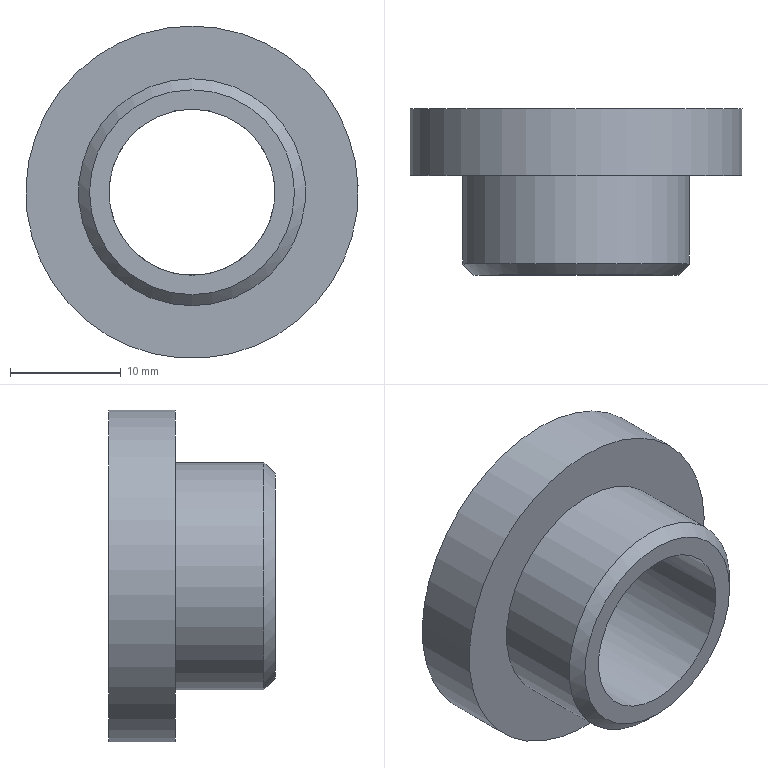Part | STEP file | HL4GZ-1.58.105 (cane-lifter cylinder pin bushing) | 1 solid | 8 faces | box 30 x 15 x 30 mm | volume 4505 mm3 | cylinder 3 | plane 3 | cone 2 | commonest cylinder face diameters 15 x1 20.5 x1 30 x1
STEP:
#1=CARTESIAN_POINT('',(0.,0.,0.));
#2=DIRECTION('',(0.,0.,1.));
#3=DIRECTION('',(1.,0.,0.));
#4=AXIS2_PLACEMENT_3D('',#1,#2,#3);
#5=CARTESIAN_POINT('',(3259.883,-564.,17.811));
#6=VERTEX_POINT('',#5);
#7=CARTESIAN_POINT('',(3259.883,-564.,10.311));
#8=DIRECTION('',(0.000001603,1.,0.000002068));
#9=DIRECTION('',(0.,-0.000002068,1.));
#10=AXIS2_PLACEMENT_3D('',#7,#8,#9);
#11=CIRCLE('',#10,7.5);
#12=CARTESIAN_POINT('',(3259.883,-564.,10.311));
#13=DIRECTION('',(0.000001603,1.,0.000002068));
#14=DIRECTION('',(0.,0.000002068,-1.));
#15=AXIS2_PLACEMENT_3D('',#12,#13,#14);
#16=CONICAL_SURFACE('',#15,7.5,0.7854);
#17=CARTESIAN_POINT('',(3.142,0.));
#18=DIRECTION('',(1.,0.));
#19=VECTOR('',#18,1.);
#20=LINE('',#17,#19);
#21=(GEOMETRIC_REPRESENTATION_CONTEXT(2)PARAMETRIC_REPRESENTATION_CONTEXT()REPRESENTATION_CONTEXT('',''));
#22=DEFINITIONAL_REPRESENTATION('',(#20),#21);
#23=PCURVE('',#16,#22);
#24=CARTESIAN_POINT('',(3259.883,-563.,10.311));
#25=DIRECTION('',(-0.000001603,-1.,-0.000002068));
#26=DIRECTION('',(0.,-0.000002068,1.));
#27=AXIS2_PLACEMENT_3D('',#24,#25,#26);
#28=CYLINDRICAL_SURFACE('',#27,7.5);
#29=CARTESIAN_POINT('',(6.283,1.));
#30=DIRECTION('',(-1.,0.));
#31=VECTOR('',#30,1.);
#32=LINE('',#29,#31);
#33=(GEOMETRIC_REPRESENTATION_CONTEXT(2)PARAMETRIC_REPRESENTATION_CONTEXT()REPRESENTATION_CONTEXT('',''));
#34=DEFINITIONAL_REPRESENTATION('',(#32),#33);
#35=PCURVE('',#28,#34);
#36=SURFACE_CURVE('',#11,(#23,#35),.PCURVE_S1.);
#37=EDGE_CURVE('',#6,#6,#36,.T.);
#38=ORIENTED_EDGE('',*,*,#37,.T.);
#39=CARTESIAN_POINT('',(3259.883,-563.,18.811));
#40=VERTEX_POINT('',#39);
#41=CARTESIAN_POINT('',(3259.883,-564.,17.811));
#42=CARTESIAN_POINT('',(3259.883,-563.,18.811));
#43=B_SPLINE_CURVE_WITH_KNOTS('',1,(#41,#42),.UNSPECIFIED.,.F.,.F.,(2,2),(0.,1.414),.PIECEWISE_BEZIER_KNOTS.);
#44=CARTESIAN_POINT('',(9.425,0.));
#45=DIRECTION('',(0.,1.));
#46=VECTOR('',#45,1.);
#47=LINE('',#44,#46);
#48=(GEOMETRIC_REPRESENTATION_CONTEXT(2)PARAMETRIC_REPRESENTATION_CONTEXT()REPRESENTATION_CONTEXT('',''));
#49=DEFINITIONAL_REPRESENTATION('',(#47),#48);
#50=PCURVE('',#16,#49);
#51=CARTESIAN_POINT('',(3.142,0.));
#52=DIRECTION('',(0.,1.));
#53=VECTOR('',#52,1.);
#54=LINE('',#51,#53);
#55=(GEOMETRIC_REPRESENTATION_CONTEXT(2)PARAMETRIC_REPRESENTATION_CONTEXT()REPRESENTATION_CONTEXT('',''));
#56=DEFINITIONAL_REPRESENTATION('',(#54),#55);
#57=PCURVE('',#16,#56);
#58=SEAM_CURVE('',#43,(#50,#57),.PCURVE_S1.);
#59=EDGE_CURVE('',#6,#40,#58,.T.);
#60=ORIENTED_EDGE('',*,*,#59,.T.);
#61=CARTESIAN_POINT('',(3259.883,-563.,10.311));
#62=DIRECTION('',(-0.000001603,-1.,-0.000002068));
#63=DIRECTION('',(0.,-0.000002068,1.));
#64=AXIS2_PLACEMENT_3D('',#61,#62,#63);
#65=CIRCLE('',#64,8.5);
#66=CARTESIAN_POINT('',(9.425,1.));
#67=DIRECTION('',(-1.,0.));
#68=VECTOR('',#67,1.);
#69=LINE('',#66,#68);
#70=(GEOMETRIC_REPRESENTATION_CONTEXT(2)PARAMETRIC_REPRESENTATION_CONTEXT()REPRESENTATION_CONTEXT('',''));
#71=DEFINITIONAL_REPRESENTATION('',(#69),#70);
#72=PCURVE('',#16,#71);
#73=CARTESIAN_POINT('',(3259.883,-563.,10.311));
#74=DIRECTION('',(0.000001603,1.,0.000002068));
#75=DIRECTION('',(0.,0.000002068,-1.));
#76=AXIS2_PLACEMENT_3D('',#73,#74,#75);
#77=PLANE('',#76);
#78=CARTESIAN_POINT('',(-8.5,0.));
#79=CARTESIAN_POINT('',(-8.5,14.722));
#80=CARTESIAN_POINT('',(4.25,7.361));
#81=CARTESIAN_POINT('',(17.,0.));
#82=CARTESIAN_POINT('',(4.25,-7.361));
#83=CARTESIAN_POINT('',(-8.5,-14.722));
#84=CARTESIAN_POINT('',(-8.5,0.));
#85=(BOUNDED_CURVE()B_SPLINE_CURVE(2,(#78,#79,#80,#81,#82,#83,#84),.UNSPECIFIED.,.T.,.F.)B_SPLINE_CURVE_WITH_KNOTS((1,2,2,2,2,1),(-2.094,0.,2.094,4.189,6.283,8.378),.UNSPECIFIED.)CURVE()GEOMETRIC_REPRESENTATION_ITEM()RATIONAL_B_SPLINE_CURVE((1.,0.5,1.,0.5,1.,0.5,1.))REPRESENTATION_ITEM(''));
#86=(GEOMETRIC_REPRESENTATION_CONTEXT(2)PARAMETRIC_REPRESENTATION_CONTEXT()REPRESENTATION_CONTEXT('',''));
#87=DEFINITIONAL_REPRESENTATION('',(#85),#86);
#88=PCURVE('',#77,#87);
#89=SURFACE_CURVE('',#65,(#72,#88),.PCURVE_S1.);
#90=EDGE_CURVE('',#40,#40,#89,.T.);
#91=ORIENTED_EDGE('',*,*,#90,.T.);
#92=ORIENTED_EDGE('',*,*,#59,.F.);
#93=EDGE_LOOP('',(#38,#60,#91,#92));
#94=FACE_BOUND('',#93,.F.);
#95=ADVANCED_FACE('',(#94),#16,.F.);
#96=CARTESIAN_POINT('',(3259.883,-577.,0.06076));
#97=VERTEX_POINT('',#96);
#98=CARTESIAN_POINT('',(3259.883,-577.,10.311));
#99=DIRECTION('',(0.000001603,1.,0.000002068));
#100=DIRECTION('',(0.,0.000002068,-1.));
#101=AXIS2_PLACEMENT_3D('',#98,#99,#100);
#102=CIRCLE('',#101,10.25);
#103=CARTESIAN_POINT('',(3259.883,-577.,10.311));
#104=DIRECTION('',(0.000001603,1.,0.000002068));
#105=DIRECTION('',(0.,0.000002068,-1.));
#106=AXIS2_PLACEMENT_3D('',#103,#104,#105);
#107=CONICAL_SURFACE('',#106,10.25,0.7854);
#108=CARTESIAN_POINT('',(0.,0.));
#109=DIRECTION('',(1.,0.));
#110=VECTOR('',#109,1.);
#111=LINE('',#108,#110);
#112=(GEOMETRIC_REPRESENTATION_CONTEXT(2)PARAMETRIC_REPRESENTATION_CONTEXT()REPRESENTATION_CONTEXT('',''));
#113=DEFINITIONAL_REPRESENTATION('',(#111),#112);
#114=PCURVE('',#107,#113);
#115=CARTESIAN_POINT('',(3259.883,-579.,10.311));
#116=DIRECTION('',(0.000001603,1.,0.000002068));
#117=DIRECTION('',(0.7903,0.,-0.6127));
#118=AXIS2_PLACEMENT_3D('',#115,#116,#117);
#119=CYLINDRICAL_SURFACE('',#118,10.25);
#120=CARTESIAN_POINT('',(0.9114,2.));
#121=DIRECTION('',(1.,0.));
#122=VECTOR('',#121,1.);
#123=LINE('',#120,#122);
#124=(GEOMETRIC_REPRESENTATION_CONTEXT(2)PARAMETRIC_REPRESENTATION_CONTEXT()REPRESENTATION_CONTEXT('',''));
#125=DEFINITIONAL_REPRESENTATION('',(#123),#124);
#126=PCURVE('',#119,#125);
#127=SURFACE_CURVE('',#102,(#114,#126),.PCURVE_S1.);
#128=EDGE_CURVE('',#97,#97,#127,.T.);
#129=ORIENTED_EDGE('',*,*,#128,.F.);
#130=CARTESIAN_POINT('',(3259.883,-578.,1.061));
#131=VERTEX_POINT('',#130);
#132=CARTESIAN_POINT('',(3259.883,-578.,1.061));
#133=CARTESIAN_POINT('',(3259.883,-577.,0.06076));
#134=B_SPLINE_CURVE_WITH_KNOTS('',1,(#132,#133),.UNSPECIFIED.,.F.,.F.,(2,2),(-1.414,0.),.PIECEWISE_BEZIER_KNOTS.);
#135=CARTESIAN_POINT('',(0.,0.));
#136=DIRECTION('',(0.,1.));
#137=VECTOR('',#136,1.);
#138=LINE('',#135,#137);
#139=(GEOMETRIC_REPRESENTATION_CONTEXT(2)PARAMETRIC_REPRESENTATION_CONTEXT()REPRESENTATION_CONTEXT('',''));
#140=DEFINITIONAL_REPRESENTATION('',(#138),#139);
#141=PCURVE('',#107,#140);
#142=CARTESIAN_POINT('',(6.283,0.));
#143=DIRECTION('',(0.,1.));
#144=VECTOR('',#143,1.);
#145=LINE('',#142,#144);
#146=(GEOMETRIC_REPRESENTATION_CONTEXT(2)PARAMETRIC_REPRESENTATION_CONTEXT()REPRESENTATION_CONTEXT('',''));
#147=DEFINITIONAL_REPRESENTATION('',(#145),#146);
#148=PCURVE('',#107,#147);
#149=SEAM_CURVE('',#134,(#141,#148),.PCURVE_S1.);
#150=EDGE_CURVE('',#131,#97,#149,.T.);
#151=ORIENTED_EDGE('',*,*,#150,.F.);
#152=CARTESIAN_POINT('',(3259.883,-578.,10.311));
#153=DIRECTION('',(-0.000001603,-1.,-0.000002068));
#154=DIRECTION('',(0.,0.000002068,-1.));
#155=AXIS2_PLACEMENT_3D('',#152,#153,#154);
#156=CIRCLE('',#155,9.25);
#157=CARTESIAN_POINT('',(6.283,-1.));
#158=DIRECTION('',(-1.,0.));
#159=VECTOR('',#158,1.);
#160=LINE('',#157,#159);
#161=(GEOMETRIC_REPRESENTATION_CONTEXT(2)PARAMETRIC_REPRESENTATION_CONTEXT()REPRESENTATION_CONTEXT('',''));
#162=DEFINITIONAL_REPRESENTATION('',(#160),#161);
#163=PCURVE('',#107,#162);
#164=CARTESIAN_POINT('',(3259.883,-578.,10.311));
#165=DIRECTION('',(-0.000001603,-1.,-0.000002068));
#166=DIRECTION('',(0.,-0.000002068,1.));
#167=AXIS2_PLACEMENT_3D('',#164,#165,#166);
#168=PLANE('',#167);
#169=CARTESIAN_POINT('',(0.,0.));
#170=DIRECTION('',(-1.,0.));
#171=AXIS2_PLACEMENT_2D('',#169,#170);
#172=CIRCLE('',#171,9.25);
#173=(GEOMETRIC_REPRESENTATION_CONTEXT(2)PARAMETRIC_REPRESENTATION_CONTEXT()REPRESENTATION_CONTEXT('',''));
#174=DEFINITIONAL_REPRESENTATION('',(#172),#173);
#175=PCURVE('',#168,#174);
#176=SURFACE_CURVE('',#156,(#163,#175),.PCURVE_S1.);
#177=EDGE_CURVE('',#131,#131,#176,.T.);
#178=ORIENTED_EDGE('',*,*,#177,.F.);
#179=ORIENTED_EDGE('',*,*,#150,.T.);
#180=EDGE_LOOP('',(#129,#151,#178,#179));
#181=FACE_BOUND('',#180,.T.);
#182=ADVANCED_FACE('',(#181),#107,.T.);
#183=CARTESIAN_POINT('',(3259.883,-569.,0.06078));
#184=VERTEX_POINT('',#183);
#185=CARTESIAN_POINT('',(3259.883,-569.,20.561));
#186=VERTEX_POINT('',#185);
#187=CARTESIAN_POINT('',(3259.883,-569.,10.311));
#188=DIRECTION('',(0.000001603,1.,0.000002068));
#189=DIRECTION('',(0.,-0.000002068,1.));
#190=AXIS2_PLACEMENT_3D('',#187,#188,#189);
#191=CIRCLE('',#190,10.25);
#192=CARTESIAN_POINT('',(-2.23,10.));
#193=DIRECTION('',(1.,0.));
#194=VECTOR('',#193,1.);
#195=LINE('',#192,#194);
#196=(GEOMETRIC_REPRESENTATION_CONTEXT(2)PARAMETRIC_REPRESENTATION_CONTEXT()REPRESENTATION_CONTEXT('',''));
#197=DEFINITIONAL_REPRESENTATION('',(#195),#196);
#198=PCURVE('',#119,#197);
#199=CARTESIAN_POINT('',(3259.883,-569.,10.311));
#200=DIRECTION('',(0.000001603,1.,0.000002068));
#201=DIRECTION('',(0.,0.000002068,-1.));
#202=AXIS2_PLACEMENT_3D('',#199,#200,#201);
#203=PLANE('',#202);
#204=CARTESIAN_POINT('',(0.,0.));
#205=DIRECTION('',(-1.,0.));
#206=AXIS2_PLACEMENT_2D('',#204,#205);
#207=CIRCLE('',#206,10.25);
#208=(GEOMETRIC_REPRESENTATION_CONTEXT(2)PARAMETRIC_REPRESENTATION_CONTEXT()REPRESENTATION_CONTEXT('',''));
#209=DEFINITIONAL_REPRESENTATION('',(#207),#208);
#210=PCURVE('',#203,#209);
#211=SURFACE_CURVE('',#191,(#198,#210),.PCURVE_S1.);
#212=EDGE_CURVE('',#184,#186,#211,.T.);
#213=ORIENTED_EDGE('',*,*,#212,.F.);
#214=CARTESIAN_POINT('',(3259.883,-577.,0.06076));
#215=CARTESIAN_POINT('',(3259.883,-569.,0.06078));
#216=B_SPLINE_CURVE_WITH_KNOTS('',1,(#214,#215),.UNSPECIFIED.,.F.,.F.,(2,2),(2.,10.),.PIECEWISE_BEZIER_KNOTS.);
#217=CARTESIAN_POINT('',(0.9114,0.));
#218=DIRECTION('',(0.,1.));
#219=VECTOR('',#218,1.);
#220=LINE('',#217,#219);
#221=(GEOMETRIC_REPRESENTATION_CONTEXT(2)PARAMETRIC_REPRESENTATION_CONTEXT()REPRESENTATION_CONTEXT('',''));
#222=DEFINITIONAL_REPRESENTATION('',(#220),#221);
#223=PCURVE('',#119,#222);
#224=CARTESIAN_POINT('',(7.195,0.));
#225=DIRECTION('',(0.,1.));
#226=VECTOR('',#225,1.);
#227=LINE('',#224,#226);
#228=(GEOMETRIC_REPRESENTATION_CONTEXT(2)PARAMETRIC_REPRESENTATION_CONTEXT()REPRESENTATION_CONTEXT('',''));
#229=DEFINITIONAL_REPRESENTATION('',(#227),#228);
#230=PCURVE('',#119,#229);
#231=SEAM_CURVE('',#216,(#223,#230),.PCURVE_S1.);
#232=EDGE_CURVE('',#97,#184,#231,.T.);
#233=ORIENTED_EDGE('',*,*,#232,.F.);
#234=ORIENTED_EDGE('',*,*,#128,.T.);
#235=ORIENTED_EDGE('',*,*,#232,.T.);
#236=CARTESIAN_POINT('',(3259.883,-569.,10.311));
#237=DIRECTION('',(0.000001603,1.,0.000002068));
#238=DIRECTION('',(0.,-0.000002068,1.));
#239=AXIS2_PLACEMENT_3D('',#236,#237,#238);
#240=CIRCLE('',#239,10.25);
#241=CARTESIAN_POINT('',(4.053,10.));
#242=DIRECTION('',(1.,0.));
#243=VECTOR('',#242,1.);
#244=LINE('',#241,#243);
#245=(GEOMETRIC_REPRESENTATION_CONTEXT(2)PARAMETRIC_REPRESENTATION_CONTEXT()REPRESENTATION_CONTEXT('',''));
#246=DEFINITIONAL_REPRESENTATION('',(#244),#245);
#247=PCURVE('',#119,#246);
#248=CARTESIAN_POINT('',(0.,0.));
#249=DIRECTION('',(-1.,0.));
#250=AXIS2_PLACEMENT_2D('',#248,#249);
#251=CIRCLE('',#250,10.25);
#252=(GEOMETRIC_REPRESENTATION_CONTEXT(2)PARAMETRIC_REPRESENTATION_CONTEXT()REPRESENTATION_CONTEXT('',''));
#253=DEFINITIONAL_REPRESENTATION('',(#251),#252);
#254=PCURVE('',#203,#253);
#255=SURFACE_CURVE('',#240,(#247,#254),.PCURVE_S1.);
#256=EDGE_CURVE('',#186,#184,#255,.T.);
#257=ORIENTED_EDGE('',*,*,#256,.F.);
#258=EDGE_LOOP('',(#213,#233,#234,#235,#257));
#259=FACE_BOUND('',#258,.T.);
#260=ADVANCED_FACE('',(#259),#119,.T.);
#261=CARTESIAN_POINT('',(3259.883,-578.,2.811));
#262=VERTEX_POINT('',#261);
#263=CARTESIAN_POINT('',(3259.883,-578.,17.811));
#264=VERTEX_POINT('',#263);
#265=CARTESIAN_POINT('',(3259.883,-578.,10.311));
#266=DIRECTION('',(0.000001603,1.,0.000002068));
#267=DIRECTION('',(0.,0.000002068,-1.));
#268=AXIS2_PLACEMENT_3D('',#265,#266,#267);
#269=CIRCLE('',#268,7.5);
#270=CARTESIAN_POINT('',(-7.5,0.));
#271=CARTESIAN_POINT('',(-7.5,12.99));
#272=CARTESIAN_POINT('',(3.75,6.495));
#273=CARTESIAN_POINT('',(15.,0.));
#274=CARTESIAN_POINT('',(3.75,-6.495));
#275=CARTESIAN_POINT('',(-7.5,-12.99));
#276=CARTESIAN_POINT('',(-7.5,0.));
#277=(BOUNDED_CURVE()B_SPLINE_CURVE(2,(#270,#271,#272,#273,#274,#275,#276),.UNSPECIFIED.,.T.,.F.)B_SPLINE_CURVE_WITH_KNOTS((1,2,2,2,2,1),(-2.094,0.,2.094,4.189,6.283,8.378),.UNSPECIFIED.)CURVE()GEOMETRIC_REPRESENTATION_ITEM()RATIONAL_B_SPLINE_CURVE((1.,0.5,1.,0.5,1.,0.5,1.))REPRESENTATION_ITEM(''));
#278=(GEOMETRIC_REPRESENTATION_CONTEXT(2)PARAMETRIC_REPRESENTATION_CONTEXT()REPRESENTATION_CONTEXT('',''));
#279=DEFINITIONAL_REPRESENTATION('',(#277),#278);
#280=PCURVE('',#168,#279);
#281=CARTESIAN_POINT('',(3.142,15.));
#282=DIRECTION('',(-1.,0.));
#283=VECTOR('',#282,1.);
#284=LINE('',#281,#283);
#285=(GEOMETRIC_REPRESENTATION_CONTEXT(2)PARAMETRIC_REPRESENTATION_CONTEXT()REPRESENTATION_CONTEXT('',''));
#286=DEFINITIONAL_REPRESENTATION('',(#284),#285);
#287=PCURVE('',#28,#286);
#288=SURFACE_CURVE('',#269,(#280,#287),.PCURVE_S1.);
#289=EDGE_CURVE('',#262,#264,#288,.T.);
#290=ORIENTED_EDGE('',*,*,#289,.T.);
#291=CARTESIAN_POINT('',(3259.883,-578.,10.311));
#292=DIRECTION('',(0.000001603,1.,0.000002068));
#293=DIRECTION('',(0.,0.000002068,-1.));
#294=AXIS2_PLACEMENT_3D('',#291,#292,#293);
#295=CIRCLE('',#294,7.5);
#296=CARTESIAN_POINT('',(-7.5,0.));
#297=CARTESIAN_POINT('',(-7.5,12.99));
#298=CARTESIAN_POINT('',(3.75,6.495));
#299=CARTESIAN_POINT('',(15.,0.));
#300=CARTESIAN_POINT('',(3.75,-6.495));
#301=CARTESIAN_POINT('',(-7.5,-12.99));
#302=CARTESIAN_POINT('',(-7.5,0.));
#303=(BOUNDED_CURVE()B_SPLINE_CURVE(2,(#296,#297,#298,#299,#300,#301,#302),.UNSPECIFIED.,.T.,.F.)B_SPLINE_CURVE_WITH_KNOTS((1,2,2,2,2,1),(-2.094,0.,2.094,4.189,6.283,8.378),.UNSPECIFIED.)CURVE()GEOMETRIC_REPRESENTATION_ITEM()RATIONAL_B_SPLINE_CURVE((1.,0.5,1.,0.5,1.,0.5,1.))REPRESENTATION_ITEM(''));
#304=(GEOMETRIC_REPRESENTATION_CONTEXT(2)PARAMETRIC_REPRESENTATION_CONTEXT()REPRESENTATION_CONTEXT('',''));
#305=DEFINITIONAL_REPRESENTATION('',(#303),#304);
#306=PCURVE('',#168,#305);
#307=CARTESIAN_POINT('',(9.425,15.));
#308=DIRECTION('',(-1.,0.));
#309=VECTOR('',#308,1.);
#310=LINE('',#307,#309);
#311=(GEOMETRIC_REPRESENTATION_CONTEXT(2)PARAMETRIC_REPRESENTATION_CONTEXT()REPRESENTATION_CONTEXT('',''));
#312=DEFINITIONAL_REPRESENTATION('',(#310),#311);
#313=PCURVE('',#28,#312);
#314=SURFACE_CURVE('',#295,(#306,#313),.PCURVE_S1.);
#315=EDGE_CURVE('',#264,#262,#314,.T.);
#316=ORIENTED_EDGE('',*,*,#315,.T.);
#317=EDGE_LOOP('',(#290,#316));
#318=FACE_BOUND('',#317,.T.);
#319=ORIENTED_EDGE('',*,*,#177,.T.);
#320=EDGE_LOOP('',(#319));
#321=FACE_BOUND('',#320,.T.);
#322=ADVANCED_FACE('',(#318,#321),#168,.T.);
#323=ORIENTED_EDGE('',*,*,#289,.T.);
#324=CARTESIAN_POINT('',(3259.883,-564.,17.811));
#325=CARTESIAN_POINT('',(3259.883,-578.,17.811));
#326=B_SPLINE_CURVE_WITH_KNOTS('',1,(#324,#325),.UNSPECIFIED.,.F.,.F.,(2,2),(1.,15.),.PIECEWISE_BEZIER_KNOTS.);
#327=CARTESIAN_POINT('',(0.,0.));
#328=DIRECTION('',(0.,1.));
#329=VECTOR('',#328,1.);
#330=LINE('',#327,#329);
#331=(GEOMETRIC_REPRESENTATION_CONTEXT(2)PARAMETRIC_REPRESENTATION_CONTEXT()REPRESENTATION_CONTEXT('',''));
#332=DEFINITIONAL_REPRESENTATION('',(#330),#331);
#333=PCURVE('',#28,#332);
#334=CARTESIAN_POINT('',(6.283,0.));
#335=DIRECTION('',(0.,1.));
#336=VECTOR('',#335,1.);
#337=LINE('',#334,#336);
#338=(GEOMETRIC_REPRESENTATION_CONTEXT(2)PARAMETRIC_REPRESENTATION_CONTEXT()REPRESENTATION_CONTEXT('',''));
#339=DEFINITIONAL_REPRESENTATION('',(#337),#338);
#340=PCURVE('',#28,#339);
#341=SEAM_CURVE('',#326,(#333,#340),.PCURVE_S1.);
#342=EDGE_CURVE('',#6,#264,#341,.T.);
#343=ORIENTED_EDGE('',*,*,#342,.F.);
#344=ORIENTED_EDGE('',*,*,#37,.F.);
#345=ORIENTED_EDGE('',*,*,#342,.T.);
#346=ORIENTED_EDGE('',*,*,#315,.T.);
#347=EDGE_LOOP('',(#323,#343,#344,#345,#346));
#348=FACE_BOUND('',#347,.F.);
#349=ADVANCED_FACE('',(#348),#28,.F.);
#350=CARTESIAN_POINT('',(3259.883,-569.,25.311));
#351=VERTEX_POINT('',#350);
#352=CARTESIAN_POINT('',(3259.883,-569.,10.311));
#353=DIRECTION('',(0.000001603,1.,0.000002068));
#354=DIRECTION('',(0.,-0.000002068,1.));
#355=AXIS2_PLACEMENT_3D('',#352,#353,#354);
#356=CIRCLE('',#355,15.);
#357=CARTESIAN_POINT('',(0.,0.));
#358=DIRECTION('',(-1.,0.));
#359=AXIS2_PLACEMENT_2D('',#357,#358);
#360=CIRCLE('',#359,15.);
#361=(GEOMETRIC_REPRESENTATION_CONTEXT(2)PARAMETRIC_REPRESENTATION_CONTEXT()REPRESENTATION_CONTEXT('',''));
#362=DEFINITIONAL_REPRESENTATION('',(#360),#361);
#363=PCURVE('',#203,#362);
#364=CARTESIAN_POINT('',(3259.883,-563.,10.311));
#365=DIRECTION('',(-0.000001603,-1.,-0.000002068));
#366=DIRECTION('',(0.,-0.000002068,1.));
#367=AXIS2_PLACEMENT_3D('',#364,#365,#366);
#368=CYLINDRICAL_SURFACE('',#367,15.);
#369=CARTESIAN_POINT('',(6.283,6.));
#370=DIRECTION('',(-1.,0.));
#371=VECTOR('',#370,1.);
#372=LINE('',#369,#371);
#373=(GEOMETRIC_REPRESENTATION_CONTEXT(2)PARAMETRIC_REPRESENTATION_CONTEXT()REPRESENTATION_CONTEXT('',''));
#374=DEFINITIONAL_REPRESENTATION('',(#372),#373);
#375=PCURVE('',#368,#374);
#376=SURFACE_CURVE('',#356,(#363,#375),.PCURVE_S1.);
#377=EDGE_CURVE('',#351,#351,#376,.T.);
#378=ORIENTED_EDGE('',*,*,#377,.F.);
#379=EDGE_LOOP('',(#378));
#380=FACE_BOUND('',#379,.T.);
#381=ORIENTED_EDGE('',*,*,#256,.T.);
#382=ORIENTED_EDGE('',*,*,#212,.T.);
#383=EDGE_LOOP('',(#381,#382));
#384=FACE_BOUND('',#383,.T.);
#385=ADVANCED_FACE('',(#380,#384),#203,.F.);
#386=CARTESIAN_POINT('',(3259.883,-563.,25.311));
#387=VERTEX_POINT('',#386);
#388=CARTESIAN_POINT('',(3259.883,-563.,10.311));
#389=DIRECTION('',(0.000001603,1.,0.000002068));
#390=DIRECTION('',(0.,-0.000002068,1.));
#391=AXIS2_PLACEMENT_3D('',#388,#389,#390);
#392=CIRCLE('',#391,15.);
#393=CARTESIAN_POINT('',(0.,0.));
#394=DIRECTION('',(-1.,0.));
#395=AXIS2_PLACEMENT_2D('',#393,#394);
#396=CIRCLE('',#395,15.);
#397=(GEOMETRIC_REPRESENTATION_CONTEXT(2)PARAMETRIC_REPRESENTATION_CONTEXT()REPRESENTATION_CONTEXT('',''));
#398=DEFINITIONAL_REPRESENTATION('',(#396),#397);
#399=PCURVE('',#77,#398);
#400=CARTESIAN_POINT('',(6.283,0.));
#401=DIRECTION('',(-1.,0.));
#402=VECTOR('',#401,1.);
#403=LINE('',#400,#402);
#404=(GEOMETRIC_REPRESENTATION_CONTEXT(2)PARAMETRIC_REPRESENTATION_CONTEXT()REPRESENTATION_CONTEXT('',''));
#405=DEFINITIONAL_REPRESENTATION('',(#403),#404);
#406=PCURVE('',#368,#405);
#407=SURFACE_CURVE('',#392,(#399,#406),.PCURVE_S1.);
#408=EDGE_CURVE('',#387,#387,#407,.T.);
#409=ORIENTED_EDGE('',*,*,#408,.T.);
#410=EDGE_LOOP('',(#409));
#411=FACE_BOUND('',#410,.T.);
#412=ORIENTED_EDGE('',*,*,#90,.T.);
#413=EDGE_LOOP('',(#412));
#414=FACE_BOUND('',#413,.T.);
#415=ADVANCED_FACE('',(#411,#414),#77,.T.);
#416=ORIENTED_EDGE('',*,*,#377,.T.);
#417=CARTESIAN_POINT('',(3259.883,-563.,25.311));
#418=CARTESIAN_POINT('',(3259.883,-569.,25.311));
#419=B_SPLINE_CURVE_WITH_KNOTS('',1,(#417,#418),.UNSPECIFIED.,.F.,.F.,(2,2),(0.,6.),.PIECEWISE_BEZIER_KNOTS.);
#420=CARTESIAN_POINT('',(0.,0.));
#421=DIRECTION('',(0.,1.));
#422=VECTOR('',#421,1.);
#423=LINE('',#420,#422);
#424=(GEOMETRIC_REPRESENTATION_CONTEXT(2)PARAMETRIC_REPRESENTATION_CONTEXT()REPRESENTATION_CONTEXT('',''));
#425=DEFINITIONAL_REPRESENTATION('',(#423),#424);
#426=PCURVE('',#368,#425);
#427=CARTESIAN_POINT('',(6.283,0.));
#428=DIRECTION('',(0.,1.));
#429=VECTOR('',#428,1.);
#430=LINE('',#427,#429);
#431=(GEOMETRIC_REPRESENTATION_CONTEXT(2)PARAMETRIC_REPRESENTATION_CONTEXT()REPRESENTATION_CONTEXT('',''));
#432=DEFINITIONAL_REPRESENTATION('',(#430),#431);
#433=PCURVE('',#368,#432);
#434=SEAM_CURVE('',#419,(#426,#433),.PCURVE_S1.);
#435=EDGE_CURVE('',#387,#351,#434,.T.);
#436=ORIENTED_EDGE('',*,*,#435,.F.);
#437=ORIENTED_EDGE('',*,*,#408,.F.);
#438=ORIENTED_EDGE('',*,*,#435,.T.);
#439=EDGE_LOOP('',(#416,#436,#437,#438));
#440=FACE_BOUND('',#439,.T.);
#441=ADVANCED_FACE('',(#440),#368,.T.);
#442=CLOSED_SHELL('',(#95,#182,#260,#322,#349,#385,#415,#441));
#443=MANIFOLD_SOLID_BREP('',#442);
#444=(LENGTH_UNIT()NAMED_UNIT(*)SI_UNIT(.MILLI.,.METRE.));
#445=UNCERTAINTY_MEASURE_WITH_UNIT(LENGTH_MEASURE(0.000005),#444,'','');
#446=(NAMED_UNIT(*)PLANE_ANGLE_UNIT()SI_UNIT($,.RADIAN.));
#447=(NAMED_UNIT(*)SI_UNIT($,.STERADIAN.)SOLID_ANGLE_UNIT());
#448=(GEOMETRIC_REPRESENTATION_CONTEXT(3)GLOBAL_UNCERTAINTY_ASSIGNED_CONTEXT((#445))GLOBAL_UNIT_ASSIGNED_CONTEXT((#444,#446,#447))REPRESENTATION_CONTEXT('',''));
#449=ADVANCED_BREP_SHAPE_REPRESENTATION('',(#4,#443),#448);